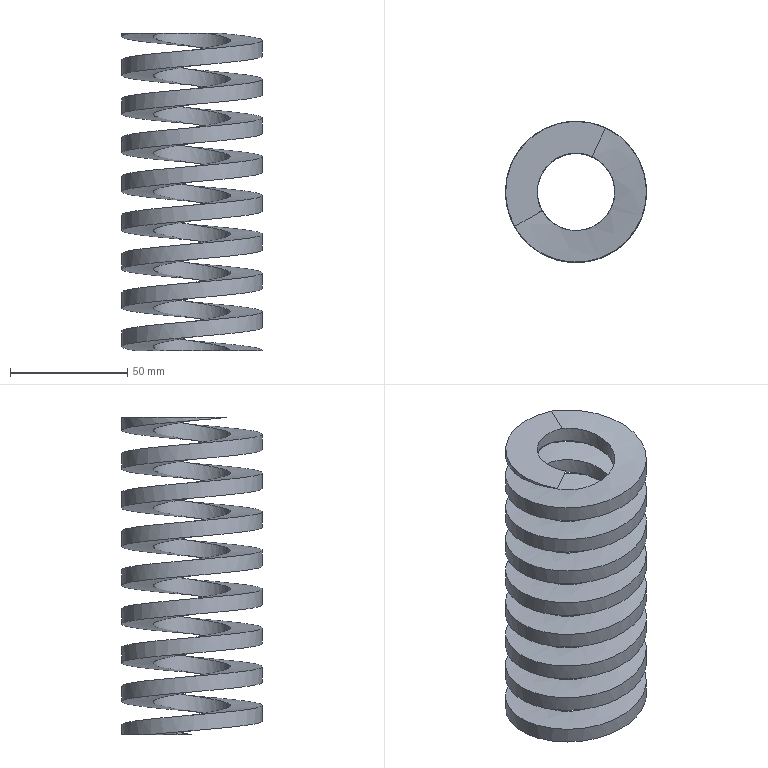Part | NX | features 模具.stp<1>[76] 2 | 1 solid | 5 faces | box 60.001 x 60 x 135.006 mm | volume 203935 mm3 | spline 2 | plane 2 | cylinder 1 | commonest cylinder face diameters 60 x1